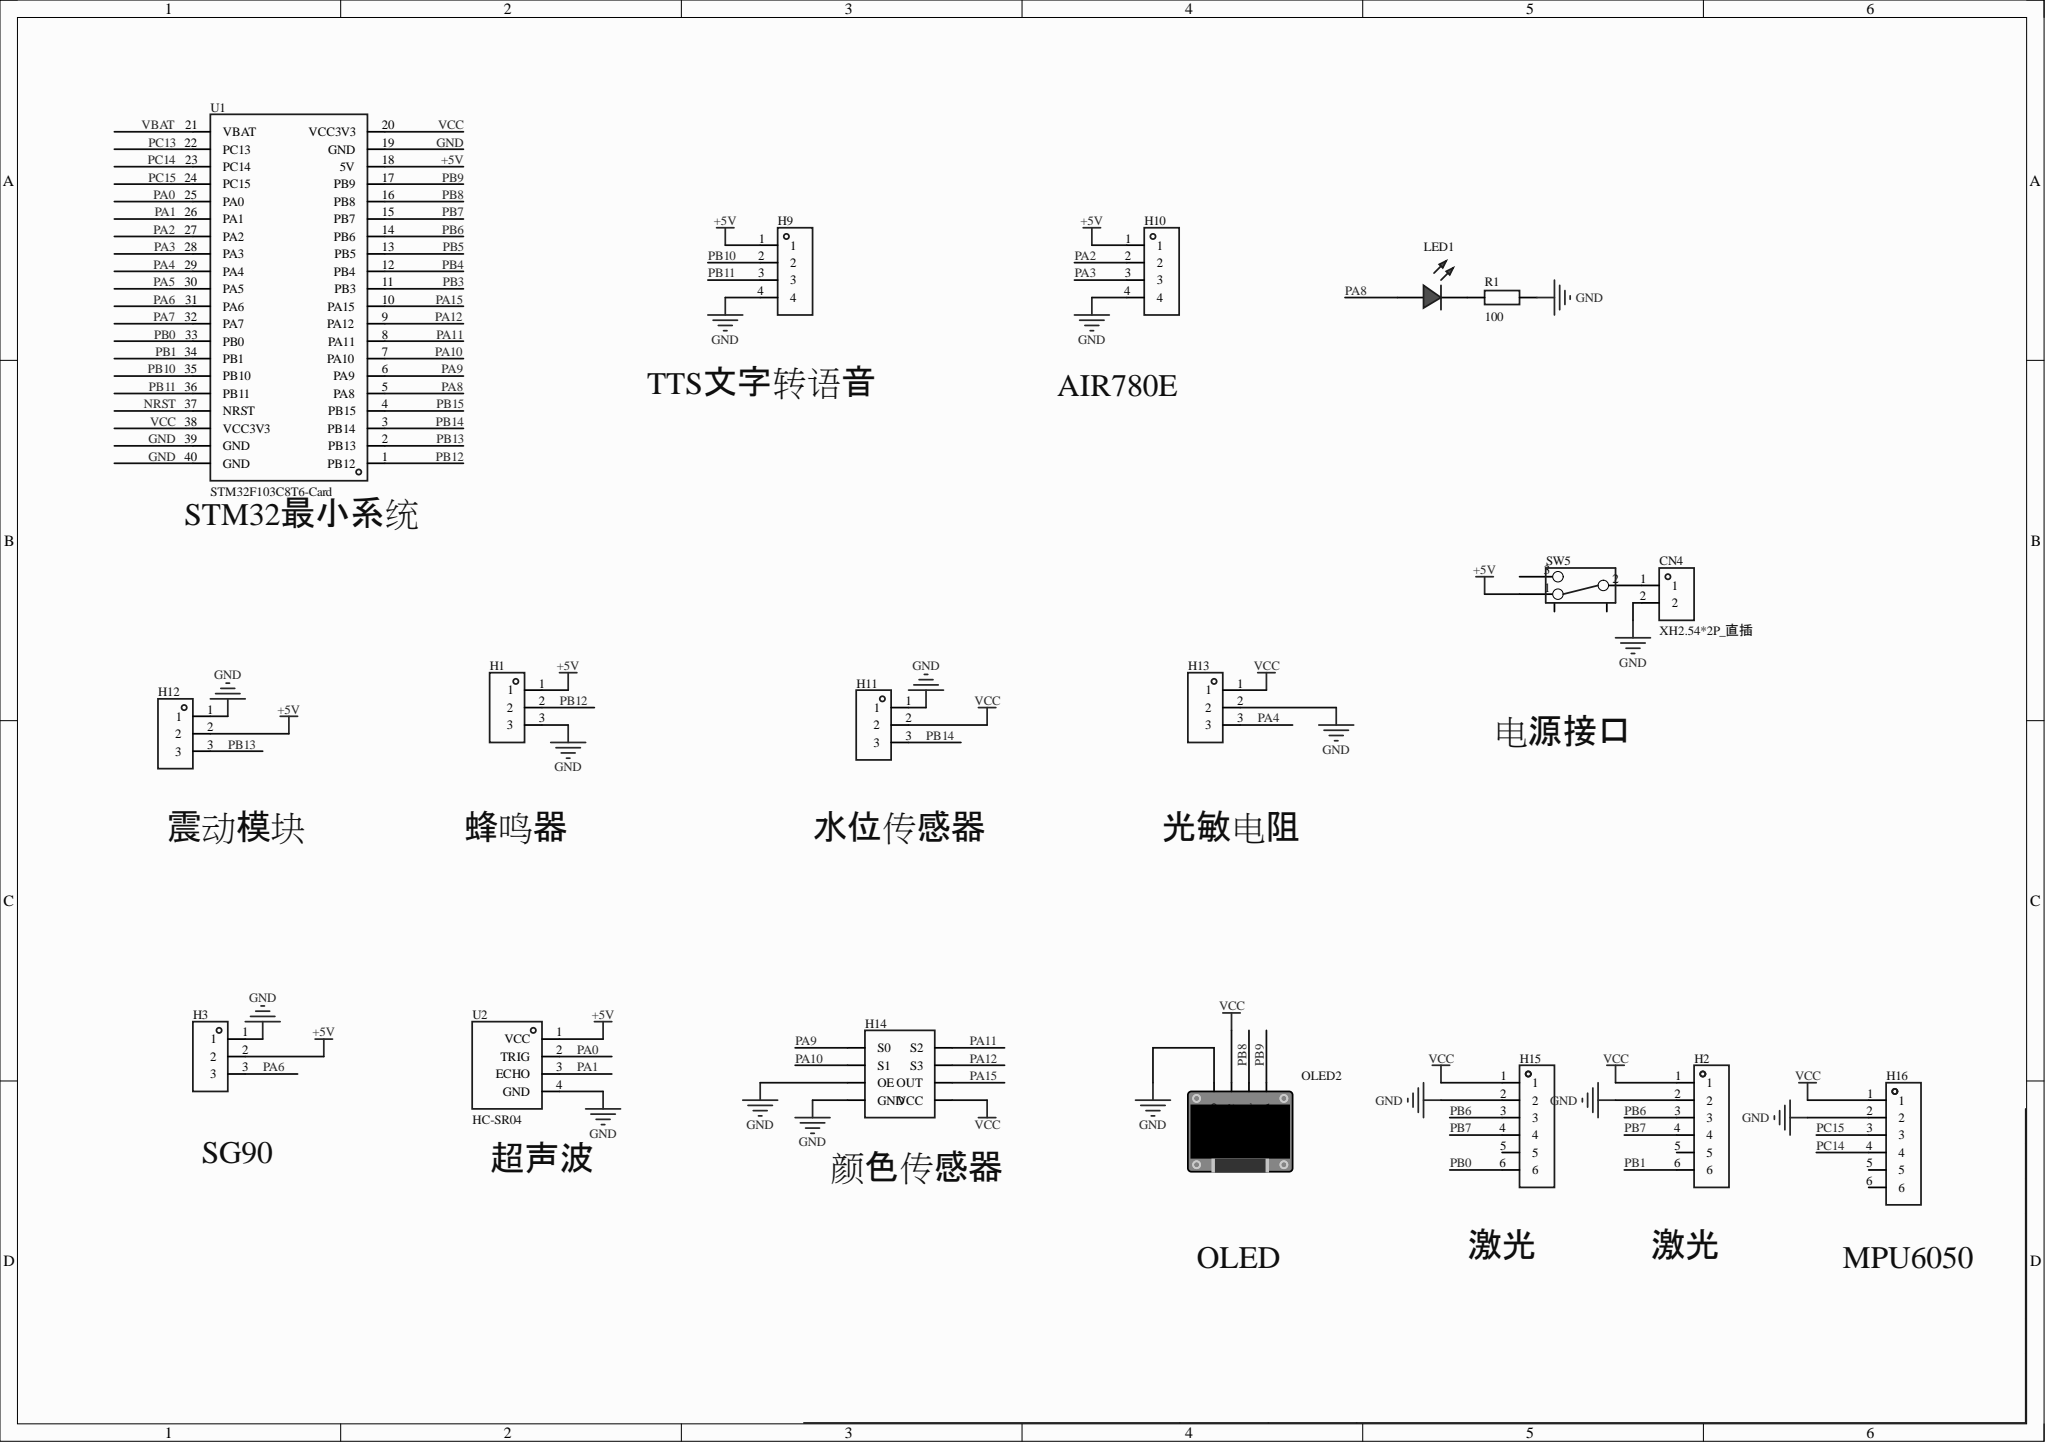Circuit board | Altium Designer | 18 parts | 30 nets
Bill of materials:
Comment,Description,Designator,Footprint,LibRef,Quantity
"XH2.54*2P_直插","","CN4","CONN-TH_2P-P2.50-XH2.54-2P","XH2.54*2P_直插","1"
"","","H1, H11, H12, H13","HDR-TH_3P-P2.54-V-F","HDR-F_2.54_1x3P","4"
"","","H2, H15, H16","HDR-TH_6P-P2.54-V-F","HDR-F_2.54_1x6P","3"
"","","H3","HDR-TH_3P-P2.54-V-M","HDR-M_2.54_1x3P","1"
"","","H9, H10","HDR-TH_4P-P2.54-V-M","HDR-M_2.54_1x4P","2"
"","","H14","HDR-TH_8P-P2.54-V-F-R2-C4-S2.54-1","HDR-F_2.54_2x4","1"
"","","LED1","LED_TH-3mm","LED_TH-R_3mm","1"
"","","OLED2","0.96OLED_4P","0.96OLED模块_4P","1"
"100","","R1","Res_1/8W","Res_AXIAL-1/8W","1"
"","","SW5","拨动开关","拨动开关_正","1"
"STM32F103C8T6-Card","","U1","CONN-TH_L53.3-W22.9_STM32F103C8T6-CARD","STM32F103C8T6-Card","1"
"HC-SR04","","U2","TH_HC-SR04V","HC-SR04","1"
Netlist (Protel format):
[
CN4
CONN-TH_2P-P2.50-XH2.54-2P
XH2.54*2P_直插



]
[
H1
HDR-TH_3P-P2.54-V-F




]
[
H2
HDR-TH_6P-P2.54-V-F




]
[
H3
HDR-TH_3P-P2.54-V-M




]
[
H9
HDR-TH_4P-P2.54-V-M




]
[
H10
HDR-TH_4P-P2.54-V-M




]
[
H11
HDR-TH_3P-P2.54-V-F




]
[
H12
HDR-TH_3P-P2.54-V-F




]
[
H13
HDR-TH_3P-P2.54-V-F




]
[
H14
HDR-TH_8P-P2.54-V-F-R2-C4-S2.54-1




]
[
H15
HDR-TH_6P-P2.54-V-F




]
[
H16
HDR-TH_6P-P2.54-V-F




]
[
LED1
LED_TH-3mm




]
[
OLED2
0.96OLED_4P




]
[
R1
Res_1/8W
100



]
[
SW5
拨动开关




]
[
U1
CONN-TH_L53.3-W22.9_STM32F103C8T6-CARD
STM32F103C8T6-Card



]
[
U2
TH_HC-SR04V
HC-SR04



]
(
VCC
H2-1
H11-2
H13-1
H14-8
H15-1
H16-1
OLED2-2
U1-20
U1-38
)
(
PC15
H16-3
U1-24
)
(
PC14
H16-4
U1-23
)
(
PB14
H11-3
U1-3
)
(
PB13
H12-3
U1-2
)
(
PB12
H1-2
U1-1
)
(
PB11
H9-3
U1-36
)
(
PB10
H9-2
U1-35
)
(
PB9
OLED2-4
U1-17
)
(
PB8
OLED2-3
U1-16
)
(
PB7
H2-4
H15-4
U1-15
)
(
PB6
H2-3
H15-3
U1-14
)
(
PB1
H2-6
U1-34
)
(
PB0
H15-6
U1-33
)
(
PA15
H14-6
U1-10
)
(
PA12
H14-4
U1-9
)
(
PA11
H14-2
U1-8
)
(
PA10
H14-3
U1-7
)
(
PA9
H14-1
U1-6
)
(
PA8
LED1-1
U1-5
)
(
PA6
H3-3
U1-31
)
(
PA4
H13-3
U1-29
)
(
PA3
H10-3
U1-28
)
(
PA2
H10-2
U1-27
)
(
PA1
U1-26
U2-3
)
(
PA0
U1-25
U2-2
)
(
NetLED1_2
LED1-2
R1-1
)
(
NetCN4_1
CN4-1
SW5-2
)
(
GND
CN4-2
H1-3
H2-2
H3-1
H9-4
H10-4
H11-1
H12-1
H13-2
H14-5
H14-7
H15-2
H16-2
OLED2-1
R1-2
U1-19
U1-39
U1-40
U2-4
)
(
+5V
H1-1
H3-2
H9-1
H10-1
H12-2
SW5-1
U1-18
U2-1
)